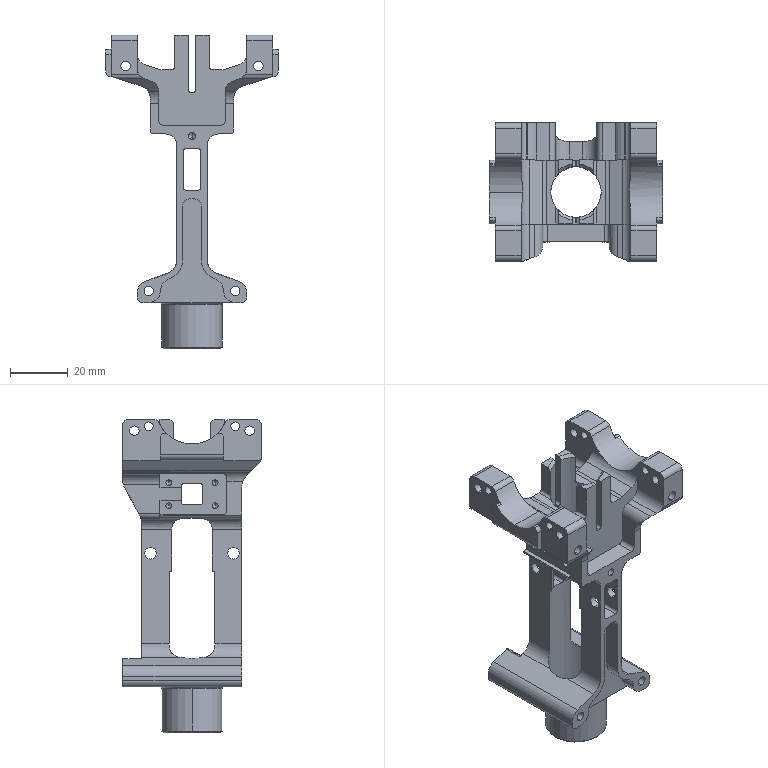Part | SolidWorks | features ICE 19, Fillet 6, HoleWzd 4, MirrorPattern 4, Chamfer 3, 3DProfileFeature 1, Extrusion 1 | 1 solid | 328 faces | box 60 x 48 x 108.75 mm | volume 35872 mm3 | cylinder 172 | plane 128 | cone 26 | spline 2 | commonest cylinder face diameters 2 x41 4 x22 8 x18 2.05 x16 3.3 x16 12 x10